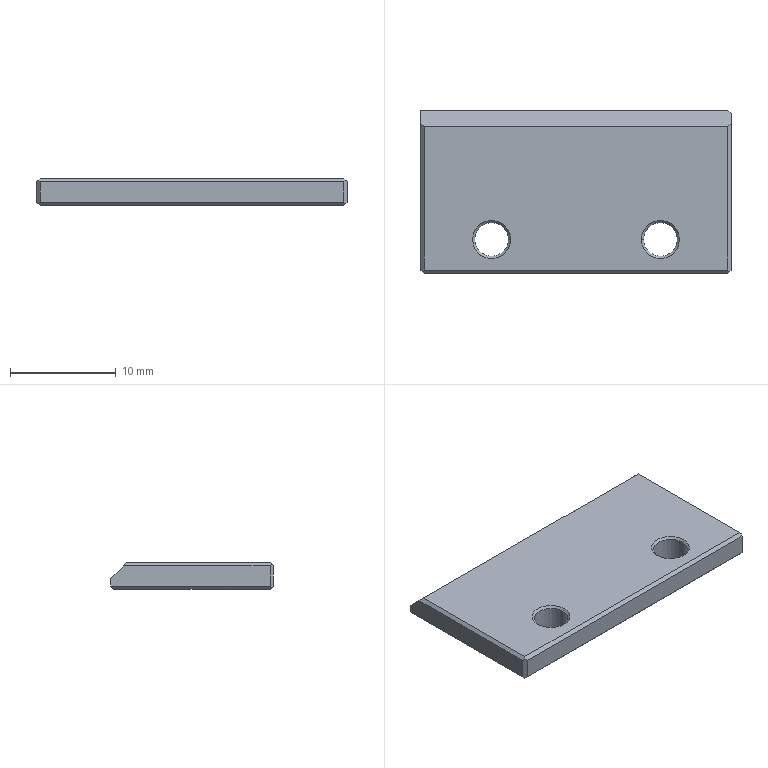Part | NX | 1 solid | 25 faces | box 29.4 x 15.4 x 2.5 mm | volume 1051 mm3 | plane 17 | cylinder 4 | cone 4 | commonest cylinder face diameters 3.2 x4
STEP:
#1=CARTESIAN_POINT('',(2038.7,121.9,62.8));
#2=VERTEX_POINT('',#1);
#3=CARTESIAN_POINT('',(2038.7,121.9,63.8));
#4=VERTEX_POINT('',#3);
#5=CARTESIAN_POINT('',(2038.7,121.9,63.75));
#6=DIRECTION('',(0.,0.,1.));
#7=VECTOR('',#6,1000.);
#8=LINE('',#5,#7);
#9=EDGE_CURVE('',#2,#4,#8,.T.);
#10=ORIENTED_EDGE('',*,*,#9,.T.);
#11=CARTESIAN_POINT('',(2038.7,121.,64.7));
#12=VERTEX_POINT('',#11);
#13=CARTESIAN_POINT('',(2038.7,123.2,62.5));
#14=DIRECTION('',(0.,-0.7071,0.7071));
#15=VECTOR('',#14,1000.);
#16=LINE('',#13,#15);
#17=EDGE_CURVE('',#4,#12,#16,.T.);
#18=ORIENTED_EDGE('',*,*,#17,.T.);
#19=CARTESIAN_POINT('',(2038.7,107.1,64.7));
#20=VERTEX_POINT('',#19);
#21=CARTESIAN_POINT('',(2038.7,114.5,64.7));
#22=DIRECTION('',(0.,-1.,0.));
#23=VECTOR('',#22,1000.);
#24=LINE('',#21,#23);
#25=EDGE_CURVE('',#12,#20,#24,.T.);
#26=ORIENTED_EDGE('',*,*,#25,.T.);
#27=CARTESIAN_POINT('',(2038.7,107.1,62.8));
#28=VERTEX_POINT('',#27);
#29=CARTESIAN_POINT('',(2038.7,107.1,63.75));
#30=DIRECTION('',(0.,0.,-1.));
#31=VECTOR('',#30,1000.);
#32=LINE('',#29,#31);
#33=EDGE_CURVE('',#20,#28,#32,.T.);
#34=ORIENTED_EDGE('',*,*,#33,.T.);
#35=CARTESIAN_POINT('',(2038.7,114.5,62.8));
#36=DIRECTION('',(0.,-1.,0.));
#37=VECTOR('',#36,1000.);
#38=LINE('',#35,#37);
#39=EDGE_CURVE('',#2,#28,#38,.T.);
#40=ORIENTED_EDGE('',*,*,#39,.F.);
#41=EDGE_LOOP('',(#10,#18,#26,#34,#40));
#42=FACE_BOUND('',#41,.T.);
#43=CARTESIAN_POINT('',(2038.7,120.2,62.5));
#44=DIRECTION('',(1.,0.,0.));
#45=DIRECTION('',(0.,1.,0.));
#46=AXIS2_PLACEMENT_3D('',#43,#44,#45);
#47=PLANE('',#46);
#48=ADVANCED_FACE('',(#42),#47,.T.);
#49=CARTESIAN_POINT('',(2038.4,122.2,62.8));
#50=VERTEX_POINT('',#49);
#51=CARTESIAN_POINT('',(2009.3,122.2,62.8));
#52=VERTEX_POINT('',#51);
#53=CARTESIAN_POINT('',(2024.,122.2,62.8));
#54=DIRECTION('',(-1.,0.,0.));
#55=VECTOR('',#54,1000.);
#56=LINE('',#53,#55);
#57=EDGE_CURVE('',#50,#52,#56,.T.);
#58=ORIENTED_EDGE('',*,*,#57,.T.);
#59=CARTESIAN_POINT('',(2009.3,122.2,63.5));
#60=VERTEX_POINT('',#59);
#61=CARTESIAN_POINT('',(2009.3,122.2,62.5));
#62=DIRECTION('',(0.,0.,-1.));
#63=VECTOR('',#62,1000.);
#64=LINE('',#61,#63);
#65=EDGE_CURVE('',#60,#52,#64,.T.);
#66=ORIENTED_EDGE('',*,*,#65,.F.);
#67=CARTESIAN_POINT('',(2038.4,122.2,63.5));
#68=VERTEX_POINT('',#67);
#69=CARTESIAN_POINT('',(2024.,122.2,63.5));
#70=DIRECTION('',(1.,0.,0.));
#71=VECTOR('',#70,1000.);
#72=LINE('',#69,#71);
#73=EDGE_CURVE('',#60,#68,#72,.T.);
#74=ORIENTED_EDGE('',*,*,#73,.T.);
#75=CARTESIAN_POINT('',(2038.4,122.2,63.75));
#76=DIRECTION('',(0.,0.,1.));
#77=VECTOR('',#76,1000.);
#78=LINE('',#75,#77);
#79=EDGE_CURVE('',#50,#68,#78,.T.);
#80=ORIENTED_EDGE('',*,*,#79,.F.);
#81=EDGE_LOOP('',(#58,#66,#74,#80));
#82=FACE_BOUND('',#81,.T.);
#83=CARTESIAN_POINT('',(2009.3,122.2,62.5));
#84=DIRECTION('',(0.,1.,0.));
#85=DIRECTION('',(1.,0.,0.));
#86=AXIS2_PLACEMENT_3D('',#83,#84,#85);
#87=PLANE('',#86);
#88=ADVANCED_FACE('',(#82),#87,.T.);
#89=CARTESIAN_POINT('',(2009.3,107.1,62.8));
#90=VERTEX_POINT('',#89);
#91=CARTESIAN_POINT('',(2009.3,107.1,64.7));
#92=VERTEX_POINT('',#91);
#93=CARTESIAN_POINT('',(2009.3,107.1,63.75));
#94=DIRECTION('',(0.,0.,1.));
#95=VECTOR('',#94,1000.);
#96=LINE('',#93,#95);
#97=EDGE_CURVE('',#90,#92,#96,.T.);
#98=ORIENTED_EDGE('',*,*,#97,.T.);
#99=CARTESIAN_POINT('',(2009.3,121.,64.7));
#100=VERTEX_POINT('',#99);
#101=CARTESIAN_POINT('',(2009.3,114.5,64.7));
#102=DIRECTION('',(0.,1.,0.));
#103=VECTOR('',#102,1000.);
#104=LINE('',#101,#103);
#105=EDGE_CURVE('',#92,#100,#104,.T.);
#106=ORIENTED_EDGE('',*,*,#105,.T.);
#107=CARTESIAN_POINT('',(2009.3,123.2,62.5));
#108=DIRECTION('',(0.,0.7071,-0.7071));
#109=VECTOR('',#108,1000.);
#110=LINE('',#107,#109);
#111=EDGE_CURVE('',#100,#60,#110,.T.);
#112=ORIENTED_EDGE('',*,*,#111,.T.);
#113=ORIENTED_EDGE('',*,*,#65,.T.);
#114=CARTESIAN_POINT('',(2009.3,114.5,62.8));
#115=DIRECTION('',(0.,1.,0.));
#116=VECTOR('',#115,1000.);
#117=LINE('',#114,#116);
#118=EDGE_CURVE('',#90,#52,#117,.T.);
#119=ORIENTED_EDGE('',*,*,#118,.F.);
#120=EDGE_LOOP('',(#98,#106,#112,#113,#119));
#121=FACE_BOUND('',#120,.T.);
#122=CARTESIAN_POINT('',(2009.3,112.8,62.5));
#123=DIRECTION('',(-1.,0.,0.));
#124=DIRECTION('',(0.,0.,1.));
#125=AXIS2_PLACEMENT_3D('',#122,#123,#124);
#126=PLANE('',#125);
#127=ADVANCED_FACE('',(#121),#126,.T.);
#128=CARTESIAN_POINT('',(2009.6,106.8,62.8));
#129=VERTEX_POINT('',#128);
#130=CARTESIAN_POINT('',(2038.4,106.8,62.8));
#131=VERTEX_POINT('',#130);
#132=CARTESIAN_POINT('',(2024.,106.8,62.8));
#133=DIRECTION('',(1.,0.,0.));
#134=VECTOR('',#133,1000.);
#135=LINE('',#132,#134);
#136=EDGE_CURVE('',#129,#131,#135,.T.);
#137=ORIENTED_EDGE('',*,*,#136,.T.);
#138=CARTESIAN_POINT('',(2038.4,106.8,64.7));
#139=VERTEX_POINT('',#138);
#140=CARTESIAN_POINT('',(2038.4,106.8,63.75));
#141=DIRECTION('',(0.,0.,-1.));
#142=VECTOR('',#141,1000.);
#143=LINE('',#140,#142);
#144=EDGE_CURVE('',#139,#131,#143,.T.);
#145=ORIENTED_EDGE('',*,*,#144,.F.);
#146=CARTESIAN_POINT('',(2009.6,106.8,64.7));
#147=VERTEX_POINT('',#146);
#148=CARTESIAN_POINT('',(2024.,106.8,64.7));
#149=DIRECTION('',(-1.,0.,0.));
#150=VECTOR('',#149,1000.);
#151=LINE('',#148,#150);
#152=EDGE_CURVE('',#139,#147,#151,.T.);
#153=ORIENTED_EDGE('',*,*,#152,.T.);
#154=CARTESIAN_POINT('',(2009.6,106.8,63.75));
#155=DIRECTION('',(0.,0.,1.));
#156=VECTOR('',#155,1000.);
#157=LINE('',#154,#156);
#158=EDGE_CURVE('',#129,#147,#157,.T.);
#159=ORIENTED_EDGE('',*,*,#158,.F.);
#160=EDGE_LOOP('',(#137,#145,#153,#159));
#161=FACE_BOUND('',#160,.T.);
#162=CARTESIAN_POINT('',(2038.7,106.8,62.5));
#163=DIRECTION('',(0.,-1.,0.));
#164=DIRECTION('',(0.,0.,-1.));
#165=AXIS2_PLACEMENT_3D('',#162,#163,#164);
#166=PLANE('',#165);
#167=ADVANCED_FACE('',(#161),#166,.T.);
#168=ORIENTED_EDGE('',*,*,#33,.F.);
#169=CARTESIAN_POINT('',(2038.55,106.95,64.85));
#170=VERTEX_POINT('',#169);
#171=CARTESIAN_POINT('',(2048.809,117.209,54.591));
#172=DIRECTION('',(-0.5774,-0.5774,0.5774));
#173=VECTOR('',#172,1000.);
#174=LINE('',#171,#173);
#175=EDGE_CURVE('',#20,#170,#174,.T.);
#176=ORIENTED_EDGE('',*,*,#175,.T.);
#177=CARTESIAN_POINT('',(2048.809,117.209,75.109));
#178=DIRECTION('',(0.5774,0.5774,0.5774));
#179=VECTOR('',#178,1000.);
#180=LINE('',#177,#179);
#181=EDGE_CURVE('',#139,#170,#180,.T.);
#182=ORIENTED_EDGE('',*,*,#181,.F.);
#183=ORIENTED_EDGE('',*,*,#144,.T.);
#184=CARTESIAN_POINT('',(2038.55,106.95,62.65));
#185=VERTEX_POINT('',#184);
#186=CARTESIAN_POINT('',(2048.809,117.209,52.391));
#187=DIRECTION('',(-0.5774,-0.5774,0.5774));
#188=VECTOR('',#187,1000.);
#189=LINE('',#186,#188);
#190=EDGE_CURVE('',#185,#131,#189,.T.);
#191=ORIENTED_EDGE('',*,*,#190,.F.);
#192=CARTESIAN_POINT('',(2048.809,117.209,72.909));
#193=DIRECTION('',(0.5774,0.5774,0.5774));
#194=VECTOR('',#193,1000.);
#195=LINE('',#192,#194);
#196=EDGE_CURVE('',#185,#28,#195,.T.);
#197=ORIENTED_EDGE('',*,*,#196,.T.);
#198=EDGE_LOOP('',(#168,#176,#182,#183,#191,#197));
#199=FACE_BOUND('',#198,.T.);
#200=CARTESIAN_POINT('',(2038.55,106.95,63.75));
#201=DIRECTION('',(0.7071,-0.7071,0.));
#202=DIRECTION('',(0.,0.,-1.));
#203=AXIS2_PLACEMENT_3D('',#200,#201,#202);
#204=PLANE('',#203);
#205=ADVANCED_FACE('',(#199),#204,.T.);
#206=ORIENTED_EDGE('',*,*,#9,.F.);
#207=CARTESIAN_POINT('',(2038.55,122.05,62.65));
#208=VERTEX_POINT('',#207);
#209=CARTESIAN_POINT('',(2043.391,117.209,67.491));
#210=DIRECTION('',(0.5774,-0.5774,0.5774));
#211=VECTOR('',#210,1000.);
#212=LINE('',#209,#211);
#213=EDGE_CURVE('',#208,#2,#212,.T.);
#214=ORIENTED_EDGE('',*,*,#213,.F.);
#215=CARTESIAN_POINT('',(2038.7,121.9,62.5));
#216=DIRECTION('',(-0.5774,0.5774,0.5774));
#217=VECTOR('',#216,1000.);
#218=LINE('',#215,#217);
#219=EDGE_CURVE('',#208,#50,#218,.T.);
#220=ORIENTED_EDGE('',*,*,#219,.T.);
#221=ORIENTED_EDGE('',*,*,#79,.T.);
#222=CARTESIAN_POINT('',(2037.4,123.2,62.5));
#223=DIRECTION('',(0.5774,-0.5774,0.5774));
#224=VECTOR('',#223,1000.);
#225=LINE('',#222,#224);
#226=EDGE_CURVE('',#68,#4,#225,.T.);
#227=ORIENTED_EDGE('',*,*,#226,.T.);
#228=EDGE_LOOP('',(#206,#214,#220,#221,#227));
#229=FACE_BOUND('',#228,.T.);
#230=CARTESIAN_POINT('',(2038.55,122.05,63.75));
#231=DIRECTION('',(0.7071,0.7071,0.));
#232=DIRECTION('',(0.,0.,-1.));
#233=AXIS2_PLACEMENT_3D('',#230,#231,#232);
#234=PLANE('',#233);
#235=ADVANCED_FACE('',(#229),#234,.T.);
#236=ORIENTED_EDGE('',*,*,#97,.F.);
#237=CARTESIAN_POINT('',(2009.45,106.95,62.65));
#238=VERTEX_POINT('',#237);
#239=CARTESIAN_POINT('',(1999.191,117.209,72.909));
#240=DIRECTION('',(-0.5774,0.5774,0.5774));
#241=VECTOR('',#240,1000.);
#242=LINE('',#239,#241);
#243=EDGE_CURVE('',#238,#90,#242,.T.);
#244=ORIENTED_EDGE('',*,*,#243,.F.);
#245=CARTESIAN_POINT('',(1999.191,117.209,52.391));
#246=DIRECTION('',(0.5774,-0.5774,0.5774));
#247=VECTOR('',#246,1000.);
#248=LINE('',#245,#247);
#249=EDGE_CURVE('',#238,#129,#248,.T.);
#250=ORIENTED_EDGE('',*,*,#249,.T.);
#251=ORIENTED_EDGE('',*,*,#158,.T.);
#252=CARTESIAN_POINT('',(2009.45,106.95,64.85));
#253=VERTEX_POINT('',#252);
#254=CARTESIAN_POINT('',(1999.191,117.209,75.109));
#255=DIRECTION('',(-0.5774,0.5774,0.5774));
#256=VECTOR('',#255,1000.);
#257=LINE('',#254,#256);
#258=EDGE_CURVE('',#147,#253,#257,.T.);
#259=ORIENTED_EDGE('',*,*,#258,.T.);
#260=CARTESIAN_POINT('',(1999.191,117.209,54.591));
#261=DIRECTION('',(0.5774,-0.5774,0.5774));
#262=VECTOR('',#261,1000.);
#263=LINE('',#260,#262);
#264=EDGE_CURVE('',#92,#253,#263,.T.);
#265=ORIENTED_EDGE('',*,*,#264,.F.);
#266=EDGE_LOOP('',(#236,#244,#250,#251,#259,#265));
#267=FACE_BOUND('',#266,.T.);
#268=CARTESIAN_POINT('',(2009.45,106.95,63.75));
#269=DIRECTION('',(-0.7071,-0.7071,0.));
#270=DIRECTION('',(-0.7071,0.7071,0.));
#271=AXIS2_PLACEMENT_3D('',#268,#269,#270);
#272=PLANE('',#271);
#273=ADVANCED_FACE('',(#267),#272,.T.);
#274=CARTESIAN_POINT('',(2009.6,120.7,65.));
#275=VERTEX_POINT('',#274);
#276=CARTESIAN_POINT('',(2038.4,120.7,65.));
#277=VERTEX_POINT('',#276);
#278=CARTESIAN_POINT('',(2024.,120.7,65.));
#279=DIRECTION('',(1.,0.,0.));
#280=VECTOR('',#279,1000.);
#281=LINE('',#278,#280);
#282=EDGE_CURVE('',#275,#277,#281,.T.);
#283=ORIENTED_EDGE('',*,*,#282,.F.);
#284=CARTESIAN_POINT('',(2009.6,107.1,65.));
#285=VERTEX_POINT('',#284);
#286=CARTESIAN_POINT('',(2009.6,114.5,65.));
#287=DIRECTION('',(0.,1.,0.));
#288=VECTOR('',#287,1000.);
#289=LINE('',#286,#288);
#290=EDGE_CURVE('',#285,#275,#289,.T.);
#291=ORIENTED_EDGE('',*,*,#290,.F.);
#292=CARTESIAN_POINT('',(2038.4,107.1,65.));
#293=VERTEX_POINT('',#292);
#294=CARTESIAN_POINT('',(2024.,107.1,65.));
#295=DIRECTION('',(-1.,0.,0.));
#296=VECTOR('',#295,1000.);
#297=LINE('',#294,#296);
#298=EDGE_CURVE('',#293,#285,#297,.T.);
#299=ORIENTED_EDGE('',*,*,#298,.F.);
#300=CARTESIAN_POINT('',(2038.4,114.5,65.));
#301=DIRECTION('',(0.,-1.,0.));
#302=VECTOR('',#301,1000.);
#303=LINE('',#300,#302);
#304=EDGE_CURVE('',#277,#293,#303,.T.);
#305=ORIENTED_EDGE('',*,*,#304,.F.);
#306=EDGE_LOOP('',(#283,#291,#299,#305));
#307=FACE_BOUND('',#306,.T.);
#308=CARTESIAN_POINT('',(2014.2,110.,65.));
#309=VERTEX_POINT('',#308);
#310=CARTESIAN_POINT('',(2017.8,110.,65.));
#311=VERTEX_POINT('',#310);
#312=CARTESIAN_POINT('',(2016.,110.,65.));
#313=DIRECTION('',(0.,0.,1.));
#314=DIRECTION('',(1.,0.,0.));
#315=AXIS2_PLACEMENT_3D('',#312,#313,#314);
#316=CIRCLE('',#315,1.8);
#317=EDGE_CURVE('',#309,#311,#316,.T.);
#318=ORIENTED_EDGE('',*,*,#317,.F.);
#319=CARTESIAN_POINT('',(2016.,110.,65.));
#320=DIRECTION('',(0.,0.,1.));
#321=DIRECTION('',(1.,0.,0.));
#322=AXIS2_PLACEMENT_3D('',#319,#320,#321);
#323=CIRCLE('',#322,1.8);
#324=EDGE_CURVE('',#311,#309,#323,.T.);
#325=ORIENTED_EDGE('',*,*,#324,.F.);
#326=EDGE_LOOP('',(#318,#325));
#327=FACE_BOUND('',#326,.T.);
#328=CARTESIAN_POINT('',(2030.2,110.,65.));
#329=VERTEX_POINT('',#328);
#330=CARTESIAN_POINT('',(2033.8,110.,65.));
#331=VERTEX_POINT('',#330);
#332=CARTESIAN_POINT('',(2032.,110.,65.));
#333=DIRECTION('',(0.,0.,1.));
#334=DIRECTION('',(1.,0.,0.));
#335=AXIS2_PLACEMENT_3D('',#332,#333,#334);
#336=CIRCLE('',#335,1.8);
#337=EDGE_CURVE('',#329,#331,#336,.T.);
#338=ORIENTED_EDGE('',*,*,#337,.F.);
#339=CARTESIAN_POINT('',(2032.,110.,65.));
#340=DIRECTION('',(0.,0.,1.));
#341=DIRECTION('',(1.,0.,0.));
#342=AXIS2_PLACEMENT_3D('',#339,#340,#341);
#343=CIRCLE('',#342,1.8);
#344=EDGE_CURVE('',#331,#329,#343,.T.);
#345=ORIENTED_EDGE('',*,*,#344,.F.);
#346=EDGE_LOOP('',(#338,#345));
#347=FACE_BOUND('',#346,.T.);
#348=CARTESIAN_POINT('',(2020.995,117.209,65.));
#349=DIRECTION('',(0.,0.,1.));
#350=DIRECTION('',(1.,0.,0.));
#351=AXIS2_PLACEMENT_3D('',#348,#349,#350);
#352=PLANE('',#351);
#353=ADVANCED_FACE('',(#307,#327,#347),#352,.T.);
#354=CARTESIAN_POINT('',(2014.4,110.,64.8));
#355=VERTEX_POINT('',#354);
#356=CARTESIAN_POINT('',(2017.6,110.,64.8));
#357=VERTEX_POINT('',#356);
#358=CARTESIAN_POINT('',(2016.,110.,64.8));
#359=DIRECTION('',(0.,0.,1.));
#360=DIRECTION('',(1.,0.,0.));
#361=AXIS2_PLACEMENT_3D('',#358,#359,#360);
#362=CIRCLE('',#361,1.6);
#363=EDGE_CURVE('',#355,#357,#362,.T.);
#364=ORIENTED_EDGE('',*,*,#363,.T.);
#365=CARTESIAN_POINT('',(2017.6,110.,62.5));
#366=VERTEX_POINT('',#365);
#367=CARTESIAN_POINT('',(2017.6,110.,65.5));
#368=DIRECTION('',(0.,0.,1.));
#369=VECTOR('',#368,1000.);
#370=LINE('',#367,#369);
#371=EDGE_CURVE('',#366,#357,#370,.T.);
#372=ORIENTED_EDGE('',*,*,#371,.F.);
#373=CARTESIAN_POINT('',(2014.4,110.,62.5));
#374=VERTEX_POINT('',#373);
#375=CARTESIAN_POINT('',(2016.,110.,62.5));
#376=DIRECTION('',(0.,0.,1.));
#377=DIRECTION('',(1.,0.,0.));
#378=AXIS2_PLACEMENT_3D('',#375,#376,#377);
#379=CIRCLE('',#378,1.6);
#380=EDGE_CURVE('',#374,#366,#379,.T.);
#381=ORIENTED_EDGE('',*,*,#380,.F.);
#382=CARTESIAN_POINT('',(2014.4,110.,65.5));
#383=DIRECTION('',(0.,0.,1.));
#384=VECTOR('',#383,1000.);
#385=LINE('',#382,#384);
#386=EDGE_CURVE('',#374,#355,#385,.T.);
#387=ORIENTED_EDGE('',*,*,#386,.T.);
#388=EDGE_LOOP('',(#364,#372,#381,#387));
#389=FACE_BOUND('',#388,.T.);
#390=CARTESIAN_POINT('',(2016.,110.,65.5));
#391=DIRECTION('',(0.,0.,1.));
#392=DIRECTION('',(1.,0.,0.));
#393=AXIS2_PLACEMENT_3D('',#390,#391,#392);
#394=CYLINDRICAL_SURFACE('',#393,1.6);
#395=ADVANCED_FACE('',(#389),#394,.F.);
#396=CARTESIAN_POINT('',(2030.4,110.,64.8));
#397=VERTEX_POINT('',#396);
#398=CARTESIAN_POINT('',(2033.6,110.,64.8));
#399=VERTEX_POINT('',#398);
#400=CARTESIAN_POINT('',(2032.,110.,64.8));
#401=DIRECTION('',(0.,0.,1.));
#402=DIRECTION('',(1.,0.,0.));
#403=AXIS2_PLACEMENT_3D('',#400,#401,#402);
#404=CIRCLE('',#403,1.6);
#405=EDGE_CURVE('',#397,#399,#404,.T.);
#406=ORIENTED_EDGE('',*,*,#405,.T.);
#407=CARTESIAN_POINT('',(2033.6,110.,62.5));
#408=VERTEX_POINT('',#407);
#409=CARTESIAN_POINT('',(2033.6,110.,65.5));
#410=DIRECTION('',(0.,0.,1.));
#411=VECTOR('',#410,1000.);
#412=LINE('',#409,#411);
#413=EDGE_CURVE('',#408,#399,#412,.T.);
#414=ORIENTED_EDGE('',*,*,#413,.F.);
#415=CARTESIAN_POINT('',(2030.4,110.,62.5));
#416=VERTEX_POINT('',#415);
#417=CARTESIAN_POINT('',(2032.,110.,62.5));
#418=DIRECTION('',(0.,0.,1.));
#419=DIRECTION('',(1.,0.,0.));
#420=AXIS2_PLACEMENT_3D('',#417,#418,#419);
#421=CIRCLE('',#420,1.6);
#422=EDGE_CURVE('',#416,#408,#421,.T.);
#423=ORIENTED_EDGE('',*,*,#422,.F.);
#424=CARTESIAN_POINT('',(2030.4,110.,65.5));
#425=DIRECTION('',(0.,0.,1.));
#426=VECTOR('',#425,1000.);
#427=LINE('',#424,#426);
#428=EDGE_CURVE('',#416,#397,#427,.T.);
#429=ORIENTED_EDGE('',*,*,#428,.T.);
#430=EDGE_LOOP('',(#406,#414,#423,#429));
#431=FACE_BOUND('',#430,.T.);
#432=CARTESIAN_POINT('',(2032.,110.,65.5));
#433=DIRECTION('',(0.,0.,1.));
#434=DIRECTION('',(1.,0.,0.));
#435=AXIS2_PLACEMENT_3D('',#432,#433,#434);
#436=CYLINDRICAL_SURFACE('',#435,1.6);
#437=ADVANCED_FACE('',(#431),#436,.F.);
#438=ORIENTED_EDGE('',*,*,#363,.F.);
#439=CARTESIAN_POINT('',(2014.4,110.,64.8));
#440=DIRECTION('',(-0.7071,0.,0.7071));
#441=VECTOR('',#440,1000.);
#442=LINE('',#439,#441);
#443=EDGE_CURVE('',#355,#309,#442,.T.);
#444=ORIENTED_EDGE('',*,*,#443,.T.);
#445=ORIENTED_EDGE('',*,*,#317,.T.);
#446=CARTESIAN_POINT('',(2017.6,110.,64.8));
#447=DIRECTION('',(0.7071,0.,0.7071));
#448=VECTOR('',#447,1000.);
#449=LINE('',#446,#448);
#450=EDGE_CURVE('',#357,#311,#449,.T.);
#451=ORIENTED_EDGE('',*,*,#450,.F.);
#452=EDGE_LOOP('',(#438,#444,#445,#451));
#453=FACE_BOUND('',#452,.T.);
#454=CARTESIAN_POINT('',(2016.,110.,64.8));
#455=DIRECTION('',(0.,0.,1.));
#456=DIRECTION('',(1.,0.,0.));
#457=AXIS2_PLACEMENT_3D('',#454,#455,#456);
#458=CONICAL_SURFACE('',#457,1.6,0.7854);
#459=ADVANCED_FACE('',(#453),#458,.F.);
#460=ORIENTED_EDGE('',*,*,#405,.F.);
#461=CARTESIAN_POINT('',(2030.4,110.,64.8));
#462=DIRECTION('',(-0.7071,0.,0.7071));
#463=VECTOR('',#462,1000.);
#464=LINE('',#461,#463);
#465=EDGE_CURVE('',#397,#329,#464,.T.);
#466=ORIENTED_EDGE('',*,*,#465,.T.);
#467=ORIENTED_EDGE('',*,*,#337,.T.);
#468=CARTESIAN_POINT('',(2033.6,110.,64.8));
#469=DIRECTION('',(0.7071,0.,0.7071));
#470=VECTOR('',#469,1000.);
#471=LINE('',#468,#470);
#472=EDGE_CURVE('',#399,#331,#471,.T.);
#473=ORIENTED_EDGE('',*,*,#472,.F.);
#474=EDGE_LOOP('',(#460,#466,#467,#473));
#475=FACE_BOUND('',#474,.T.);
#476=CARTESIAN_POINT('',(2032.,110.,64.8));
#477=DIRECTION('',(0.,0.,1.));
#478=DIRECTION('',(1.,0.,0.));
#479=AXIS2_PLACEMENT_3D('',#476,#477,#478);
#480=CONICAL_SURFACE('',#479,1.6,0.7854);
#481=ADVANCED_FACE('',(#475),#480,.F.);
#482=ORIENTED_EDGE('',*,*,#304,.T.);
#483=CARTESIAN_POINT('',(2028.291,117.209,75.109));
#484=DIRECTION('',(0.5774,-0.5774,-0.5774));
#485=VECTOR('',#484,1000.);
#486=LINE('',#483,#485);
#487=EDGE_CURVE('',#293,#170,#486,.T.);
#488=ORIENTED_EDGE('',*,*,#487,.T.);
#489=ORIENTED_EDGE('',*,*,#175,.F.);
#490=ORIENTED_EDGE('',*,*,#25,.F.);
#491=CARTESIAN_POINT('',(2020.995,103.295,82.405));
#492=DIRECTION('',(0.5774,0.5774,-0.5774));
#493=VECTOR('',#492,1000.);
#494=LINE('',#491,#493);
#495=EDGE_CURVE('',#277,#12,#494,.T.);
#496=ORIENTED_EDGE('',*,*,#495,.F.);
#497=EDGE_LOOP('',(#482,#488,#489,#490,#496));
#498=FACE_BOUND('',#497,.T.);
#499=CARTESIAN_POINT('',(2038.55,114.5,64.85));
#500=DIRECTION('',(-0.7071,0.,-0.7071));
#501=DIRECTION('',(-0.7071,0.,0.7071));
#502=AXIS2_PLACEMENT_3D('',#499,#500,#501);
#503=PLANE('',#502);
#504=ADVANCED_FACE('',(#498),#503,.F.);
#505=ORIENTED_EDGE('',*,*,#298,.T.);
#506=CARTESIAN_POINT('',(2019.709,117.209,75.109));
#507=DIRECTION('',(-0.5774,-0.5774,-0.5774));
#508=VECTOR('',#507,1000.);
#509=LINE('',#506,#508);
#510=EDGE_CURVE('',#285,#253,#509,.T.);
#511=ORIENTED_EDGE('',*,*,#510,.T.);
#512=ORIENTED_EDGE('',*,*,#258,.F.);
#513=ORIENTED_EDGE('',*,*,#152,.F.);
#514=ORIENTED_EDGE('',*,*,#181,.T.);
#515=ORIENTED_EDGE('',*,*,#487,.F.);
#516=EDGE_LOOP('',(#505,#511,#512,#513,#514,#515));
#517=FACE_BOUND('',#516,.T.);
#518=CARTESIAN_POINT('',(2024.,106.95,64.85));
#519=DIRECTION('',(0.,0.7071,-0.7071));
#520=DIRECTION('',(-1.,0.,0.));
#521=AXIS2_PLACEMENT_3D('',#518,#519,#520);
#522=PLANE('',#521);
#523=ADVANCED_FACE('',(#517),#522,.F.);
#524=ORIENTED_EDGE('',*,*,#290,.T.);
#525=CARTESIAN_POINT('',(2020.995,109.305,76.395));
#526=DIRECTION('',(0.5774,-0.5774,0.5774));
#527=VECTOR('',#526,1000.);
#528=LINE('',#525,#527);
#529=EDGE_CURVE('',#100,#275,#528,.T.);
#530=ORIENTED_EDGE('',*,*,#529,.F.);
#531=ORIENTED_EDGE('',*,*,#105,.F.);
#532=ORIENTED_EDGE('',*,*,#264,.T.);
#533=ORIENTED_EDGE('',*,*,#510,.F.);
#534=EDGE_LOOP('',(#524,#530,#531,#532,#533));
#535=FACE_BOUND('',#534,.T.);
#536=CARTESIAN_POINT('',(2009.45,114.5,64.85));
#537=DIRECTION('',(0.7071,0.,-0.7071));
#538=DIRECTION('',(0.,-1.,0.));
#539=AXIS2_PLACEMENT_3D('',#536,#537,#538);
#540=PLANE('',#539);
#541=ADVANCED_FACE('',(#535),#540,.F.);
#542=ORIENTED_EDGE('',*,*,#282,.T.);
#543=ORIENTED_EDGE('',*,*,#495,.T.);
#544=ORIENTED_EDGE('',*,*,#17,.F.);
#545=ORIENTED_EDGE('',*,*,#226,.F.);
#546=ORIENTED_EDGE('',*,*,#73,.F.);
#547=ORIENTED_EDGE('',*,*,#111,.F.);
#548=ORIENTED_EDGE('',*,*,#529,.T.);
#549=EDGE_LOOP('',(#542,#543,#544,#545,#546,#547,#548));
#550=FACE_BOUND('',#549,.T.);
#551=CARTESIAN_POINT('',(2024.,121.45,64.25));
#552=DIRECTION('',(0.,-0.7071,-0.7071));
#553=DIRECTION('',(0.,-0.7071,0.7071));
#554=AXIS2_PLACEMENT_3D('',#551,#552,#553);
#555=PLANE('',#554);
#556=ADVANCED_FACE('',(#550),#555,.F.);
#557=ORIENTED_EDGE('',*,*,#413,.T.);
#558=CARTESIAN_POINT('',(2032.,110.,64.8));
#559=DIRECTION('',(0.,0.,1.));
#560=DIRECTION('',(1.,0.,0.));
#561=AXIS2_PLACEMENT_3D('',#558,#559,#560);
#562=CIRCLE('',#561,1.6);
#563=EDGE_CURVE('',#399,#397,#562,.T.);
#564=ORIENTED_EDGE('',*,*,#563,.T.);
#565=ORIENTED_EDGE('',*,*,#428,.F.);
#566=CARTESIAN_POINT('',(2032.,110.,62.5));
#567=DIRECTION('',(0.,0.,1.));
#568=DIRECTION('',(1.,0.,0.));
#569=AXIS2_PLACEMENT_3D('',#566,#567,#568);
#570=CIRCLE('',#569,1.6);
#571=EDGE_CURVE('',#408,#416,#570,.T.);
#572=ORIENTED_EDGE('',*,*,#571,.F.);
#573=EDGE_LOOP('',(#557,#564,#565,#572));
#574=FACE_BOUND('',#573,.T.);
#575=CARTESIAN_POINT('',(2032.,110.,65.5));
#576=DIRECTION('',(0.,0.,1.));
#577=DIRECTION('',(1.,0.,0.));
#578=AXIS2_PLACEMENT_3D('',#575,#576,#577);
#579=CYLINDRICAL_SURFACE('',#578,1.6);
#580=ADVANCED_FACE('',(#574),#579,.F.);
#581=ORIENTED_EDGE('',*,*,#472,.T.);
#582=ORIENTED_EDGE('',*,*,#344,.T.);
#583=ORIENTED_EDGE('',*,*,#465,.F.);
#584=ORIENTED_EDGE('',*,*,#563,.F.);
#585=EDGE_LOOP('',(#581,#582,#583,#584));
#586=FACE_BOUND('',#585,.T.);
#587=CARTESIAN_POINT('',(2032.,110.,64.8));
#588=DIRECTION('',(0.,0.,1.));
#589=DIRECTION('',(1.,0.,0.));
#590=AXIS2_PLACEMENT_3D('',#587,#588,#589);
#591=CONICAL_SURFACE('',#590,1.6,0.7854);
#592=ADVANCED_FACE('',(#586),#591,.F.);
#593=ORIENTED_EDGE('',*,*,#371,.T.);
#594=CARTESIAN_POINT('',(2016.,110.,64.8));
#595=DIRECTION('',(0.,0.,1.));
#596=DIRECTION('',(1.,0.,0.));
#597=AXIS2_PLACEMENT_3D('',#594,#595,#596);
#598=CIRCLE('',#597,1.6);
#599=EDGE_CURVE('',#357,#355,#598,.T.);
#600=ORIENTED_EDGE('',*,*,#599,.T.);
#601=ORIENTED_EDGE('',*,*,#386,.F.);
#602=CARTESIAN_POINT('',(2016.,110.,62.5));
#603=DIRECTION('',(0.,0.,1.));
#604=DIRECTION('',(1.,0.,0.));
#605=AXIS2_PLACEMENT_3D('',#602,#603,#604);
#606=CIRCLE('',#605,1.6);
#607=EDGE_CURVE('',#366,#374,#606,.T.);
#608=ORIENTED_EDGE('',*,*,#607,.F.);
#609=EDGE_LOOP('',(#593,#600,#601,#608));
#610=FACE_BOUND('',#609,.T.);
#611=CARTESIAN_POINT('',(2016.,110.,65.5));
#612=DIRECTION('',(0.,0.,1.));
#613=DIRECTION('',(1.,0.,0.));
#614=AXIS2_PLACEMENT_3D('',#611,#612,#613);
#615=CYLINDRICAL_SURFACE('',#614,1.6);
#616=ADVANCED_FACE('',(#610),#615,.F.);
#617=ORIENTED_EDGE('',*,*,#450,.T.);
#618=ORIENTED_EDGE('',*,*,#324,.T.);
#619=ORIENTED_EDGE('',*,*,#443,.F.);
#620=ORIENTED_EDGE('',*,*,#599,.F.);
#621=EDGE_LOOP('',(#617,#618,#619,#620));
#622=FACE_BOUND('',#621,.T.);
#623=CARTESIAN_POINT('',(2016.,110.,64.8));
#624=DIRECTION('',(0.,0.,1.));
#625=DIRECTION('',(1.,0.,0.));
#626=AXIS2_PLACEMENT_3D('',#623,#624,#625);
#627=CONICAL_SURFACE('',#626,1.6,0.7854);
#628=ADVANCED_FACE('',(#622),#627,.F.);
#629=CARTESIAN_POINT('',(2009.6,107.1,62.5));
#630=VERTEX_POINT('',#629);
#631=CARTESIAN_POINT('',(2009.6,121.9,62.5));
#632=VERTEX_POINT('',#631);
#633=CARTESIAN_POINT('',(2009.6,114.5,62.5));
#634=DIRECTION('',(0.,1.,0.));
#635=VECTOR('',#634,1000.);
#636=LINE('',#633,#635);
#637=EDGE_CURVE('',#630,#632,#636,.T.);
#638=ORIENTED_EDGE('',*,*,#637,.T.);
#639=CARTESIAN_POINT('',(2038.4,121.9,62.5));
#640=VERTEX_POINT('',#639);
#641=CARTESIAN_POINT('',(2024.,121.9,62.5));
#642=DIRECTION('',(-1.,0.,0.));
#643=VECTOR('',#642,1000.);
#644=LINE('',#641,#643);
#645=EDGE_CURVE('',#640,#632,#644,.T.);
#646=ORIENTED_EDGE('',*,*,#645,.F.);
#647=CARTESIAN_POINT('',(2038.4,107.1,62.5));
#648=VERTEX_POINT('',#647);
#649=CARTESIAN_POINT('',(2038.4,114.5,62.5));
#650=DIRECTION('',(0.,-1.,0.));
#651=VECTOR('',#650,1000.);
#652=LINE('',#649,#651);
#653=EDGE_CURVE('',#640,#648,#652,.T.);
#654=ORIENTED_EDGE('',*,*,#653,.T.);
#655=CARTESIAN_POINT('',(2024.,107.1,62.5));
#656=DIRECTION('',(1.,0.,0.));
#657=VECTOR('',#656,1000.);
#658=LINE('',#655,#657);
#659=EDGE_CURVE('',#630,#648,#658,.T.);
#660=ORIENTED_EDGE('',*,*,#659,.F.);
#661=EDGE_LOOP('',(#638,#646,#654,#660));
#662=FACE_BOUND('',#661,.T.);
#663=ORIENTED_EDGE('',*,*,#380,.T.);
#664=ORIENTED_EDGE('',*,*,#607,.T.);
#665=EDGE_LOOP('',(#663,#664));
#666=FACE_BOUND('',#665,.T.);
#667=ORIENTED_EDGE('',*,*,#422,.T.);
#668=ORIENTED_EDGE('',*,*,#571,.T.);
#669=EDGE_LOOP('',(#667,#668));
#670=FACE_BOUND('',#669,.T.);
#671=CARTESIAN_POINT('',(2020.995,117.209,62.5));
#672=DIRECTION('',(0.,0.,1.));
#673=DIRECTION('',(1.,0.,0.));
#674=AXIS2_PLACEMENT_3D('',#671,#672,#673);
#675=PLANE('',#674);
#676=ADVANCED_FACE('',(#662,#666,#670),#675,.F.);
#677=ORIENTED_EDGE('',*,*,#659,.T.);
#678=CARTESIAN_POINT('',(2028.291,117.209,52.391));
#679=DIRECTION('',(-0.5774,0.5774,-0.5774));
#680=VECTOR('',#679,1000.);
#681=LINE('',#678,#680);
#682=EDGE_CURVE('',#185,#648,#681,.T.);
#683=ORIENTED_EDGE('',*,*,#682,.F.);
#684=ORIENTED_EDGE('',*,*,#190,.T.);
#685=ORIENTED_EDGE('',*,*,#136,.F.);
#686=ORIENTED_EDGE('',*,*,#249,.F.);
#687=CARTESIAN_POINT('',(2019.709,117.209,52.391));
#688=DIRECTION('',(-0.5774,-0.5774,0.5774));
#689=VECTOR('',#688,1000.);
#690=LINE('',#687,#689);
#691=EDGE_CURVE('',#630,#238,#690,.T.);
#692=ORIENTED_EDGE('',*,*,#691,.F.);
#693=EDGE_LOOP('',(#677,#683,#684,#685,#686,#692));
#694=FACE_BOUND('',#693,.T.);
#695=CARTESIAN_POINT('',(2024.,106.95,62.65));
#696=DIRECTION('',(0.,0.7071,0.7071));
#697=DIRECTION('',(1.,0.,0.));
#698=AXIS2_PLACEMENT_3D('',#695,#696,#697);
#699=PLANE('',#698);
#700=ADVANCED_FACE('',(#694),#699,.F.);
#701=ORIENTED_EDGE('',*,*,#653,.F.);
#702=CARTESIAN_POINT('',(2020.995,104.495,45.095));
#703=DIRECTION('',(-0.5774,-0.5774,-0.5774));
#704=VECTOR('',#703,1000.);
#705=LINE('',#702,#704);
#706=EDGE_CURVE('',#208,#640,#705,.T.);
#707=ORIENTED_EDGE('',*,*,#706,.F.);
#708=ORIENTED_EDGE('',*,*,#213,.T.);
#709=ORIENTED_EDGE('',*,*,#39,.T.);
#710=ORIENTED_EDGE('',*,*,#196,.F.);
#711=ORIENTED_EDGE('',*,*,#682,.T.);
#712=EDGE_LOOP('',(#701,#707,#708,#709,#710,#711));
#713=FACE_BOUND('',#712,.T.);
#714=CARTESIAN_POINT('',(2038.55,114.5,62.65));
#715=DIRECTION('',(0.7071,0.,-0.7071));
#716=DIRECTION('',(0.,-1.,0.));
#717=AXIS2_PLACEMENT_3D('',#714,#715,#716);
#718=PLANE('',#717);
#719=ADVANCED_FACE('',(#713),#718,.T.);
#720=ORIENTED_EDGE('',*,*,#645,.T.);
#721=CARTESIAN_POINT('',(2020.995,110.505,51.105));
#722=DIRECTION('',(0.5774,-0.5774,-0.5774));
#723=VECTOR('',#722,1000.);
#724=LINE('',#721,#723);
#725=EDGE_CURVE('',#52,#632,#724,.T.);
#726=ORIENTED_EDGE('',*,*,#725,.F.);
#727=ORIENTED_EDGE('',*,*,#57,.F.);
#728=ORIENTED_EDGE('',*,*,#219,.F.);
#729=ORIENTED_EDGE('',*,*,#706,.T.);
#730=EDGE_LOOP('',(#720,#726,#727,#728,#729));
#731=FACE_BOUND('',#730,.T.);
#732=CARTESIAN_POINT('',(2024.,122.05,62.65));
#733=DIRECTION('',(0.,-0.7071,0.7071));
#734=DIRECTION('',(-1.,0.,0.));
#735=AXIS2_PLACEMENT_3D('',#732,#733,#734);
#736=PLANE('',#735);
#737=ADVANCED_FACE('',(#731),#736,.F.);
#738=ORIENTED_EDGE('',*,*,#637,.F.);
#739=ORIENTED_EDGE('',*,*,#691,.T.);
#740=ORIENTED_EDGE('',*,*,#243,.T.);
#741=ORIENTED_EDGE('',*,*,#118,.T.);
#742=ORIENTED_EDGE('',*,*,#725,.T.);
#743=EDGE_LOOP('',(#738,#739,#740,#741,#742));
#744=FACE_BOUND('',#743,.T.);
#745=CARTESIAN_POINT('',(2009.45,114.5,62.65));
#746=DIRECTION('',(-0.7071,0.,-0.7071));
#747=DIRECTION('',(-0.7071,0.,0.7071));
#748=AXIS2_PLACEMENT_3D('',#745,#746,#747);
#749=PLANE('',#748);
#750=ADVANCED_FACE('',(#744),#749,.T.);
#751=CLOSED_SHELL('',(#48,#88,#127,#167,#205,#235,#273,#353,#395,#437,#459,#481,#504,#523,#541,#556,#580,#592,#616,#628,#676,#700,#719,#737,#750));
#752=MANIFOLD_SOLID_BREP('',#751);
#753=(LENGTH_UNIT()NAMED_UNIT(*)SI_UNIT(.MILLI.,.METRE.));
#754=UNCERTAINTY_MEASURE_WITH_UNIT(LENGTH_MEASURE(0.00001),#753,'','');
#755=(NAMED_UNIT(*)PLANE_ANGLE_UNIT()SI_UNIT($,.RADIAN.));
#756=(NAMED_UNIT(*)SI_UNIT($,.STERADIAN.)SOLID_ANGLE_UNIT());
#757=(GEOMETRIC_REPRESENTATION_CONTEXT(3)GLOBAL_UNCERTAINTY_ASSIGNED_CONTEXT((#754))GLOBAL_UNIT_ASSIGNED_CONTEXT((#753,#755,#756))REPRESENTATION_CONTEXT('',''));
#758=ADVANCED_BREP_SHAPE_REPRESENTATION('',(#752),#757);